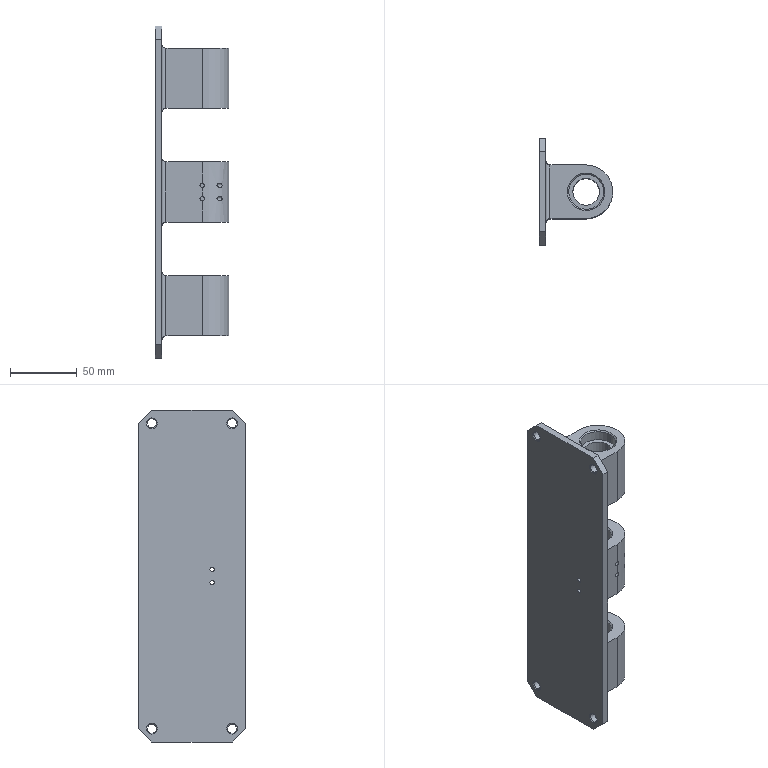Part | STEP file | Lower hinge plate thickness 20 widened | 1 solid | 93 faces | box 55 x 80 x 248 mm | volume 298124 mm3 | cylinder 49 | plane 24 | cone 20 | commonest cylinder face diameters 3.3 x16 6 x12 6.8 x8 20 x6 26 x4 40 x3